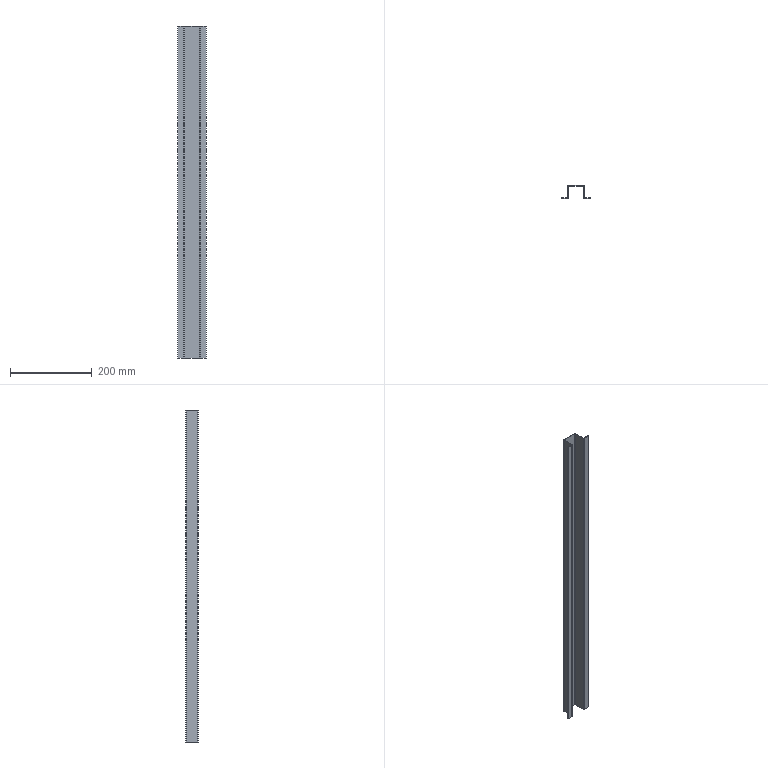Part | SolidWorks | features BaseBody 1 | 1 solid | 38 faces | box 70 x 31 x 812 mm | volume 103469 mm3 | plane 30 | cylinder 8 | commonest cylinder face diameters 2 x4 4 x4
STEP:
#1=CARTESIAN_POINT('',(41.,-1.,-406.));
#2=VERTEX_POINT('',#1);
#3=CARTESIAN_POINT('',(55.,-1.,-406.));
#4=VERTEX_POINT('',#3);
#5=CARTESIAN_POINT('',(40.,-1.,-406.));
#6=DIRECTION('',(1.,0.,0.));
#7=VECTOR('',#6,1000.);
#8=LINE('',#5,#7);
#9=EDGE_CURVE('',#2,#4,#8,.T.);
#10=ORIENTED_EDGE('',*,*,#9,.F.);
#11=CARTESIAN_POINT('',(41.,0.,-406.));
#12=VERTEX_POINT('',#11);
#13=CARTESIAN_POINT('',(41.,-1.,-406.));
#14=DIRECTION('',(0.,1.,0.));
#15=VECTOR('',#14,1000.);
#16=LINE('',#13,#15);
#17=EDGE_CURVE('',#2,#12,#16,.T.);
#18=ORIENTED_EDGE('',*,*,#17,.T.);
#19=CARTESIAN_POINT('',(55.,0.,-406.));
#20=VERTEX_POINT('',#19);
#21=CARTESIAN_POINT('',(40.,0.,-406.));
#22=DIRECTION('',(1.,0.,0.));
#23=VECTOR('',#22,1000.);
#24=LINE('',#21,#23);
#25=EDGE_CURVE('',#12,#20,#24,.T.);
#26=ORIENTED_EDGE('',*,*,#25,.T.);
#27=CARTESIAN_POINT('',(55.,0.,-406.));
#28=DIRECTION('',(0.,-1.,0.));
#29=VECTOR('',#28,1000.);
#30=LINE('',#27,#29);
#31=EDGE_CURVE('',#20,#4,#30,.T.);
#32=ORIENTED_EDGE('',*,*,#31,.T.);
#33=EDGE_LOOP('',(#10,#18,#26,#32));
#34=FACE_OUTER_BOUND('',#33,.T.);
#35=CARTESIAN_POINT('',(41.,1.,-406.));
#36=DIRECTION('',(0.,0.,-1.));
#37=DIRECTION('',(0.,-1.,0.));
#38=AXIS2_PLACEMENT_3D('',#35,#36,#37);
#39=PLANE('',#38);
#40=ADVANCED_FACE('',(#34),#39,.T.);
#41=CARTESIAN_POINT('',(-15.,-1.,406.));
#42=VERTEX_POINT('',#41);
#43=CARTESIAN_POINT('',(-1.,-1.,406.));
#44=VERTEX_POINT('',#43);
#45=CARTESIAN_POINT('',(0.,-1.,406.));
#46=DIRECTION('',(1.,0.,0.));
#47=VECTOR('',#46,1000.);
#48=LINE('',#45,#47);
#49=EDGE_CURVE('',#42,#44,#48,.T.);
#50=ORIENTED_EDGE('',*,*,#49,.T.);
#51=CARTESIAN_POINT('',(-1.,0.,406.));
#52=VERTEX_POINT('',#51);
#53=CARTESIAN_POINT('',(-1.,-1.,406.));
#54=DIRECTION('',(0.,1.,0.));
#55=VECTOR('',#54,1000.);
#56=LINE('',#53,#55);
#57=EDGE_CURVE('',#44,#52,#56,.T.);
#58=ORIENTED_EDGE('',*,*,#57,.T.);
#59=CARTESIAN_POINT('',(-15.,0.,406.));
#60=VERTEX_POINT('',#59);
#61=CARTESIAN_POINT('',(0.,0.,406.));
#62=DIRECTION('',(1.,0.,0.));
#63=VECTOR('',#62,1000.);
#64=LINE('',#61,#63);
#65=EDGE_CURVE('',#60,#52,#64,.T.);
#66=ORIENTED_EDGE('',*,*,#65,.F.);
#67=CARTESIAN_POINT('',(-15.,-1.,406.));
#68=DIRECTION('',(0.,1.,0.));
#69=VECTOR('',#68,1000.);
#70=LINE('',#67,#69);
#71=EDGE_CURVE('',#42,#60,#70,.T.);
#72=ORIENTED_EDGE('',*,*,#71,.F.);
#73=EDGE_LOOP('',(#50,#58,#66,#72));
#74=FACE_OUTER_BOUND('',#73,.T.);
#75=CARTESIAN_POINT('',(41.,1.,406.));
#76=DIRECTION('',(0.,0.,-1.));
#77=DIRECTION('',(0.,-1.,0.));
#78=AXIS2_PLACEMENT_3D('',#75,#76,#77);
#79=PLANE('',#78);
#80=ADVANCED_FACE('',(#74),#79,.F.);
#81=CARTESIAN_POINT('',(39.,1.,-406.));
#82=VERTEX_POINT('',#81);
#83=CARTESIAN_POINT('',(41.,1.,-406.));
#84=DIRECTION('',(0.,0.,1.));
#85=DIRECTION('',(1.,0.,0.));
#86=AXIS2_PLACEMENT_3D('',#83,#84,#85);
#87=CIRCLE('',#86,2.);
#88=EDGE_CURVE('',#82,#2,#87,.T.);
#89=ORIENTED_EDGE('',*,*,#88,.T.);
#90=CARTESIAN_POINT('',(41.,-1.,406.));
#91=VERTEX_POINT('',#90);
#92=CARTESIAN_POINT('',(41.,-1.,406.));
#93=DIRECTION('',(0.,0.,-1.));
#94=VECTOR('',#93,1000.);
#95=LINE('',#92,#94);
#96=EDGE_CURVE('',#91,#2,#95,.T.);
#97=ORIENTED_EDGE('',*,*,#96,.F.);
#98=CARTESIAN_POINT('',(39.,1.,406.));
#99=VERTEX_POINT('',#98);
#100=CARTESIAN_POINT('',(41.,1.,406.));
#101=DIRECTION('',(0.,0.,1.));
#102=DIRECTION('',(1.,0.,0.));
#103=AXIS2_PLACEMENT_3D('',#100,#101,#102);
#104=CIRCLE('',#103,2.);
#105=EDGE_CURVE('',#99,#91,#104,.T.);
#106=ORIENTED_EDGE('',*,*,#105,.F.);
#107=CARTESIAN_POINT('',(39.,1.,406.));
#108=DIRECTION('',(0.,0.,-1.));
#109=VECTOR('',#108,1000.);
#110=LINE('',#107,#109);
#111=EDGE_CURVE('',#99,#82,#110,.T.);
#112=ORIENTED_EDGE('',*,*,#111,.T.);
#113=EDGE_LOOP('',(#89,#97,#106,#112));
#114=FACE_OUTER_BOUND('',#113,.T.);
#115=CARTESIAN_POINT('',(41.,1.,406.));
#116=DIRECTION('',(0.,0.,-1.));
#117=DIRECTION('',(-1.,0.,0.));
#118=AXIS2_PLACEMENT_3D('',#115,#116,#117);
#119=CYLINDRICAL_SURFACE('',#118,2.);
#120=ADVANCED_FACE('',(#114),#119,.T.);
#121=CARTESIAN_POINT('',(39.,28.,-406.));
#122=VERTEX_POINT('',#121);
#123=CARTESIAN_POINT('',(39.,30.,-406.));
#124=DIRECTION('',(0.,-1.,0.));
#125=VECTOR('',#124,1000.);
#126=LINE('',#123,#125);
#127=EDGE_CURVE('',#122,#82,#126,.T.);
#128=ORIENTED_EDGE('',*,*,#127,.T.);
#129=ORIENTED_EDGE('',*,*,#111,.F.);
#130=CARTESIAN_POINT('',(39.,28.,406.));
#131=VERTEX_POINT('',#130);
#132=CARTESIAN_POINT('',(39.,30.,406.));
#133=DIRECTION('',(0.,-1.,0.));
#134=VECTOR('',#133,1000.);
#135=LINE('',#132,#134);
#136=EDGE_CURVE('',#131,#99,#135,.T.);
#137=ORIENTED_EDGE('',*,*,#136,.F.);
#138=CARTESIAN_POINT('',(39.,28.,406.));
#139=DIRECTION('',(0.,0.,-1.));
#140=VECTOR('',#139,1000.);
#141=LINE('',#138,#140);
#142=EDGE_CURVE('',#131,#122,#141,.T.);
#143=ORIENTED_EDGE('',*,*,#142,.T.);
#144=EDGE_LOOP('',(#128,#129,#137,#143));
#145=FACE_OUTER_BOUND('',#144,.T.);
#146=CARTESIAN_POINT('',(39.,30.,406.));
#147=DIRECTION('',(1.,0.,0.));
#148=DIRECTION('',(0.,1.,0.));
#149=AXIS2_PLACEMENT_3D('',#146,#147,#148);
#150=PLANE('',#149);
#151=ADVANCED_FACE('',(#145),#150,.F.);
#152=CARTESIAN_POINT('',(38.,29.,-406.));
#153=VERTEX_POINT('',#152);
#154=CARTESIAN_POINT('',(38.,28.,-406.));
#155=DIRECTION('',(0.,0.,-1.));
#156=DIRECTION('',(1.,0.,0.));
#157=AXIS2_PLACEMENT_3D('',#154,#155,#156);
#158=CIRCLE('',#157,1.);
#159=EDGE_CURVE('',#153,#122,#158,.T.);
#160=ORIENTED_EDGE('',*,*,#159,.T.);
#161=ORIENTED_EDGE('',*,*,#142,.F.);
#162=CARTESIAN_POINT('',(38.,29.,406.));
#163=VERTEX_POINT('',#162);
#164=CARTESIAN_POINT('',(38.,28.,406.));
#165=DIRECTION('',(0.,0.,-1.));
#166=DIRECTION('',(1.,0.,0.));
#167=AXIS2_PLACEMENT_3D('',#164,#165,#166);
#168=CIRCLE('',#167,1.);
#169=EDGE_CURVE('',#163,#131,#168,.T.);
#170=ORIENTED_EDGE('',*,*,#169,.F.);
#171=CARTESIAN_POINT('',(38.,29.,406.));
#172=DIRECTION('',(0.,0.,-1.));
#173=VECTOR('',#172,1000.);
#174=LINE('',#171,#173);
#175=EDGE_CURVE('',#163,#153,#174,.T.);
#176=ORIENTED_EDGE('',*,*,#175,.T.);
#177=EDGE_LOOP('',(#160,#161,#170,#176));
#178=FACE_OUTER_BOUND('',#177,.T.);
#179=CARTESIAN_POINT('',(38.,28.,406.));
#180=DIRECTION('',(0.,0.,-1.));
#181=DIRECTION('',(-1.,0.,0.));
#182=AXIS2_PLACEMENT_3D('',#179,#180,#181);
#183=CYLINDRICAL_SURFACE('',#182,1.);
#184=ADVANCED_FACE('',(#178),#183,.F.);
#185=CARTESIAN_POINT('',(2.,29.,-406.));
#186=VERTEX_POINT('',#185);
#187=CARTESIAN_POINT('',(0.,29.,-406.));
#188=DIRECTION('',(1.,0.,0.));
#189=VECTOR('',#188,1000.);
#190=LINE('',#187,#189);
#191=EDGE_CURVE('',#186,#153,#190,.T.);
#192=ORIENTED_EDGE('',*,*,#191,.T.);
#193=ORIENTED_EDGE('',*,*,#175,.F.);
#194=CARTESIAN_POINT('',(2.,29.,406.));
#195=VERTEX_POINT('',#194);
#196=CARTESIAN_POINT('',(0.,29.,406.));
#197=DIRECTION('',(1.,0.,0.));
#198=VECTOR('',#197,1000.);
#199=LINE('',#196,#198);
#200=EDGE_CURVE('',#195,#163,#199,.T.);
#201=ORIENTED_EDGE('',*,*,#200,.F.);
#202=CARTESIAN_POINT('',(2.,29.,406.));
#203=DIRECTION('',(0.,0.,-1.));
#204=VECTOR('',#203,1000.);
#205=LINE('',#202,#204);
#206=EDGE_CURVE('',#195,#186,#205,.T.);
#207=ORIENTED_EDGE('',*,*,#206,.T.);
#208=EDGE_LOOP('',(#192,#193,#201,#207));
#209=FACE_OUTER_BOUND('',#208,.T.);
#210=CARTESIAN_POINT('',(0.,29.,406.));
#211=DIRECTION('',(0.,1.,0.));
#212=DIRECTION('',(1.,0.,0.));
#213=AXIS2_PLACEMENT_3D('',#210,#211,#212);
#214=PLANE('',#213);
#215=ADVANCED_FACE('',(#209),#214,.F.);
#216=CARTESIAN_POINT('',(1.,28.,-406.));
#217=VERTEX_POINT('',#216);
#218=CARTESIAN_POINT('',(2.,28.,-406.));
#219=DIRECTION('',(0.,0.,-1.));
#220=DIRECTION('',(1.,0.,0.));
#221=AXIS2_PLACEMENT_3D('',#218,#219,#220);
#222=CIRCLE('',#221,1.);
#223=EDGE_CURVE('',#217,#186,#222,.T.);
#224=ORIENTED_EDGE('',*,*,#223,.T.);
#225=ORIENTED_EDGE('',*,*,#206,.F.);
#226=CARTESIAN_POINT('',(1.,28.,406.));
#227=VERTEX_POINT('',#226);
#228=CARTESIAN_POINT('',(2.,28.,406.));
#229=DIRECTION('',(0.,0.,-1.));
#230=DIRECTION('',(1.,0.,0.));
#231=AXIS2_PLACEMENT_3D('',#228,#229,#230);
#232=CIRCLE('',#231,1.);
#233=EDGE_CURVE('',#227,#195,#232,.T.);
#234=ORIENTED_EDGE('',*,*,#233,.F.);
#235=CARTESIAN_POINT('',(1.,28.,406.));
#236=DIRECTION('',(0.,0.,-1.));
#237=VECTOR('',#236,1000.);
#238=LINE('',#235,#237);
#239=EDGE_CURVE('',#227,#217,#238,.T.);
#240=ORIENTED_EDGE('',*,*,#239,.T.);
#241=EDGE_LOOP('',(#224,#225,#234,#240));
#242=FACE_OUTER_BOUND('',#241,.T.);
#243=CARTESIAN_POINT('',(2.,28.,406.));
#244=DIRECTION('',(0.,0.,-1.));
#245=DIRECTION('',(-1.,0.,0.));
#246=AXIS2_PLACEMENT_3D('',#243,#244,#245);
#247=CYLINDRICAL_SURFACE('',#246,1.);
#248=ADVANCED_FACE('',(#242),#247,.F.);
#249=CARTESIAN_POINT('',(1.,1.,-406.));
#250=VERTEX_POINT('',#249);
#251=CARTESIAN_POINT('',(1.,0.,-406.));
#252=DIRECTION('',(0.,1.,0.));
#253=VECTOR('',#252,1000.);
#254=LINE('',#251,#253);
#255=EDGE_CURVE('',#250,#217,#254,.T.);
#256=ORIENTED_EDGE('',*,*,#255,.T.);
#257=ORIENTED_EDGE('',*,*,#239,.F.);
#258=CARTESIAN_POINT('',(1.,1.,406.));
#259=VERTEX_POINT('',#258);
#260=CARTESIAN_POINT('',(1.,0.,406.));
#261=DIRECTION('',(0.,1.,0.));
#262=VECTOR('',#261,1000.);
#263=LINE('',#260,#262);
#264=EDGE_CURVE('',#259,#227,#263,.T.);
#265=ORIENTED_EDGE('',*,*,#264,.F.);
#266=CARTESIAN_POINT('',(1.,1.,406.));
#267=DIRECTION('',(0.,0.,-1.));
#268=VECTOR('',#267,1000.);
#269=LINE('',#266,#268);
#270=EDGE_CURVE('',#259,#250,#269,.T.);
#271=ORIENTED_EDGE('',*,*,#270,.T.);
#272=EDGE_LOOP('',(#256,#257,#265,#271));
#273=FACE_OUTER_BOUND('',#272,.T.);
#274=CARTESIAN_POINT('',(1.,0.,406.));
#275=DIRECTION('',(-1.,0.,0.));
#276=DIRECTION('',(0.,0.,1.));
#277=AXIS2_PLACEMENT_3D('',#274,#275,#276);
#278=PLANE('',#277);
#279=ADVANCED_FACE('',(#273),#278,.F.);
#280=CARTESIAN_POINT('',(-1.,-1.,-406.));
#281=VERTEX_POINT('',#280);
#282=CARTESIAN_POINT('',(-1.,1.,-406.));
#283=DIRECTION('',(0.,0.,1.));
#284=DIRECTION('',(1.,0.,0.));
#285=AXIS2_PLACEMENT_3D('',#282,#283,#284);
#286=CIRCLE('',#285,2.);
#287=EDGE_CURVE('',#281,#250,#286,.T.);
#288=ORIENTED_EDGE('',*,*,#287,.T.);
#289=ORIENTED_EDGE('',*,*,#270,.F.);
#290=CARTESIAN_POINT('',(-1.,1.,406.));
#291=DIRECTION('',(0.,0.,1.));
#292=DIRECTION('',(1.,0.,0.));
#293=AXIS2_PLACEMENT_3D('',#290,#291,#292);
#294=CIRCLE('',#293,2.);
#295=EDGE_CURVE('',#44,#259,#294,.T.);
#296=ORIENTED_EDGE('',*,*,#295,.F.);
#297=CARTESIAN_POINT('',(-1.,-1.,406.));
#298=DIRECTION('',(0.,0.,-1.));
#299=VECTOR('',#298,1000.);
#300=LINE('',#297,#299);
#301=EDGE_CURVE('',#44,#281,#300,.T.);
#302=ORIENTED_EDGE('',*,*,#301,.T.);
#303=EDGE_LOOP('',(#288,#289,#296,#302));
#304=FACE_OUTER_BOUND('',#303,.T.);
#305=CARTESIAN_POINT('',(-1.,1.,406.));
#306=DIRECTION('',(0.,0.,-1.));
#307=DIRECTION('',(-1.,0.,0.));
#308=AXIS2_PLACEMENT_3D('',#305,#306,#307);
#309=CYLINDRICAL_SURFACE('',#308,2.);
#310=ADVANCED_FACE('',(#304),#309,.T.);
#311=CARTESIAN_POINT('',(-15.,-1.,-406.));
#312=VERTEX_POINT('',#311);
#313=CARTESIAN_POINT('',(0.,-1.,-406.));
#314=DIRECTION('',(1.,0.,0.));
#315=VECTOR('',#314,1000.);
#316=LINE('',#313,#315);
#317=EDGE_CURVE('',#312,#281,#316,.T.);
#318=ORIENTED_EDGE('',*,*,#317,.T.);
#319=ORIENTED_EDGE('',*,*,#301,.F.);
#320=ORIENTED_EDGE('',*,*,#49,.F.);
#321=CARTESIAN_POINT('',(-15.,-1.,406.));
#322=DIRECTION('',(0.,0.,-1.));
#323=VECTOR('',#322,1000.);
#324=LINE('',#321,#323);
#325=EDGE_CURVE('',#42,#312,#324,.T.);
#326=ORIENTED_EDGE('',*,*,#325,.T.);
#327=EDGE_LOOP('',(#318,#319,#320,#326));
#328=FACE_OUTER_BOUND('',#327,.T.);
#329=CARTESIAN_POINT('',(0.,-1.,406.));
#330=DIRECTION('',(0.,1.,0.));
#331=DIRECTION('',(1.,0.,0.));
#332=AXIS2_PLACEMENT_3D('',#329,#330,#331);
#333=PLANE('',#332);
#334=ADVANCED_FACE('',(#328),#333,.F.);
#335=CARTESIAN_POINT('',(-15.,0.,-406.));
#336=VERTEX_POINT('',#335);
#337=CARTESIAN_POINT('',(-15.,-1.,-406.));
#338=DIRECTION('',(0.,1.,0.));
#339=VECTOR('',#338,1000.);
#340=LINE('',#337,#339);
#341=EDGE_CURVE('',#312,#336,#340,.T.);
#342=ORIENTED_EDGE('',*,*,#341,.F.);
#343=ORIENTED_EDGE('',*,*,#325,.F.);
#344=ORIENTED_EDGE('',*,*,#71,.T.);
#345=CARTESIAN_POINT('',(-15.,0.,406.));
#346=DIRECTION('',(0.,0.,-1.));
#347=VECTOR('',#346,1000.);
#348=LINE('',#345,#347);
#349=EDGE_CURVE('',#60,#336,#348,.T.);
#350=ORIENTED_EDGE('',*,*,#349,.T.);
#351=EDGE_LOOP('',(#342,#343,#344,#350));
#352=FACE_OUTER_BOUND('',#351,.T.);
#353=CARTESIAN_POINT('',(-15.,-1.,406.));
#354=DIRECTION('',(-1.,0.,0.));
#355=DIRECTION('',(0.,0.,1.));
#356=AXIS2_PLACEMENT_3D('',#353,#354,#355);
#357=PLANE('',#356);
#358=ADVANCED_FACE('',(#352),#357,.T.);
#359=CARTESIAN_POINT('',(-1.,0.,-406.));
#360=VERTEX_POINT('',#359);
#361=CARTESIAN_POINT('',(0.,0.,-406.));
#362=DIRECTION('',(1.,0.,0.));
#363=VECTOR('',#362,1000.);
#364=LINE('',#361,#363);
#365=EDGE_CURVE('',#336,#360,#364,.T.);
#366=ORIENTED_EDGE('',*,*,#365,.F.);
#367=ORIENTED_EDGE('',*,*,#349,.F.);
#368=ORIENTED_EDGE('',*,*,#65,.T.);
#369=CARTESIAN_POINT('',(-1.,0.,406.));
#370=DIRECTION('',(0.,0.,-1.));
#371=VECTOR('',#370,1000.);
#372=LINE('',#369,#371);
#373=EDGE_CURVE('',#52,#360,#372,.T.);
#374=ORIENTED_EDGE('',*,*,#373,.T.);
#375=EDGE_LOOP('',(#366,#367,#368,#374));
#376=FACE_OUTER_BOUND('',#375,.T.);
#377=CARTESIAN_POINT('',(0.,0.,406.));
#378=DIRECTION('',(0.,1.,0.));
#379=DIRECTION('',(1.,0.,0.));
#380=AXIS2_PLACEMENT_3D('',#377,#378,#379);
#381=PLANE('',#380);
#382=ADVANCED_FACE('',(#376),#381,.T.);
#383=CARTESIAN_POINT('',(0.,1.,-406.));
#384=VERTEX_POINT('',#383);
#385=CARTESIAN_POINT('',(-1.,1.,-406.));
#386=DIRECTION('',(0.,0.,1.));
#387=DIRECTION('',(-1.,0.,0.));
#388=AXIS2_PLACEMENT_3D('',#385,#386,#387);
#389=CIRCLE('',#388,1.);
#390=EDGE_CURVE('',#360,#384,#389,.T.);
#391=ORIENTED_EDGE('',*,*,#390,.F.);
#392=ORIENTED_EDGE('',*,*,#373,.F.);
#393=CARTESIAN_POINT('',(0.,1.,406.));
#394=VERTEX_POINT('',#393);
#395=CARTESIAN_POINT('',(-1.,1.,406.));
#396=DIRECTION('',(0.,0.,1.));
#397=DIRECTION('',(-1.,0.,0.));
#398=AXIS2_PLACEMENT_3D('',#395,#396,#397);
#399=CIRCLE('',#398,1.);
#400=EDGE_CURVE('',#52,#394,#399,.T.);
#401=ORIENTED_EDGE('',*,*,#400,.T.);
#402=CARTESIAN_POINT('',(0.,1.,406.));
#403=DIRECTION('',(0.,0.,-1.));
#404=VECTOR('',#403,1000.);
#405=LINE('',#402,#404);
#406=EDGE_CURVE('',#394,#384,#405,.T.);
#407=ORIENTED_EDGE('',*,*,#406,.T.);
#408=EDGE_LOOP('',(#391,#392,#401,#407));
#409=FACE_OUTER_BOUND('',#408,.T.);
#410=CARTESIAN_POINT('',(-1.,1.,406.));
#411=DIRECTION('',(0.,0.,-1.));
#412=DIRECTION('',(-1.,0.,0.));
#413=AXIS2_PLACEMENT_3D('',#410,#411,#412);
#414=CYLINDRICAL_SURFACE('',#413,1.);
#415=ADVANCED_FACE('',(#409),#414,.F.);
#416=CARTESIAN_POINT('',(0.,28.,-406.));
#417=VERTEX_POINT('',#416);
#418=CARTESIAN_POINT('',(0.,0.,-406.));
#419=DIRECTION('',(0.,1.,0.));
#420=VECTOR('',#419,1000.);
#421=LINE('',#418,#420);
#422=EDGE_CURVE('',#384,#417,#421,.T.);
#423=ORIENTED_EDGE('',*,*,#422,.F.);
#424=ORIENTED_EDGE('',*,*,#406,.F.);
#425=CARTESIAN_POINT('',(0.,28.,406.));
#426=VERTEX_POINT('',#425);
#427=CARTESIAN_POINT('',(0.,0.,406.));
#428=DIRECTION('',(0.,1.,0.));
#429=VECTOR('',#428,1000.);
#430=LINE('',#427,#429);
#431=EDGE_CURVE('',#394,#426,#430,.T.);
#432=ORIENTED_EDGE('',*,*,#431,.T.);
#433=CARTESIAN_POINT('',(0.,28.,406.));
#434=DIRECTION('',(0.,0.,-1.));
#435=VECTOR('',#434,1000.);
#436=LINE('',#433,#435);
#437=EDGE_CURVE('',#426,#417,#436,.T.);
#438=ORIENTED_EDGE('',*,*,#437,.T.);
#439=EDGE_LOOP('',(#423,#424,#432,#438));
#440=FACE_OUTER_BOUND('',#439,.T.);
#441=CARTESIAN_POINT('',(0.,0.,406.));
#442=DIRECTION('',(-1.,0.,0.));
#443=DIRECTION('',(0.,0.,1.));
#444=AXIS2_PLACEMENT_3D('',#441,#442,#443);
#445=PLANE('',#444);
#446=ADVANCED_FACE('',(#440),#445,.T.);
#447=CARTESIAN_POINT('',(2.,30.,-406.));
#448=VERTEX_POINT('',#447);
#449=CARTESIAN_POINT('',(2.,28.,-406.));
#450=DIRECTION('',(0.,0.,-1.));
#451=DIRECTION('',(1.,0.,0.));
#452=AXIS2_PLACEMENT_3D('',#449,#450,#451);
#453=CIRCLE('',#452,2.);
#454=EDGE_CURVE('',#417,#448,#453,.T.);
#455=ORIENTED_EDGE('',*,*,#454,.F.);
#456=ORIENTED_EDGE('',*,*,#437,.F.);
#457=CARTESIAN_POINT('',(2.,30.,406.));
#458=VERTEX_POINT('',#457);
#459=CARTESIAN_POINT('',(2.,28.,406.));
#460=DIRECTION('',(0.,0.,-1.));
#461=DIRECTION('',(1.,0.,0.));
#462=AXIS2_PLACEMENT_3D('',#459,#460,#461);
#463=CIRCLE('',#462,2.);
#464=EDGE_CURVE('',#426,#458,#463,.T.);
#465=ORIENTED_EDGE('',*,*,#464,.T.);
#466=CARTESIAN_POINT('',(2.,30.,406.));
#467=DIRECTION('',(0.,0.,-1.));
#468=VECTOR('',#467,1000.);
#469=LINE('',#466,#468);
#470=EDGE_CURVE('',#458,#448,#469,.T.);
#471=ORIENTED_EDGE('',*,*,#470,.T.);
#472=EDGE_LOOP('',(#455,#456,#465,#471));
#473=FACE_OUTER_BOUND('',#472,.T.);
#474=CARTESIAN_POINT('',(2.,28.,406.));
#475=DIRECTION('',(0.,0.,-1.));
#476=DIRECTION('',(-1.,0.,0.));
#477=AXIS2_PLACEMENT_3D('',#474,#475,#476);
#478=CYLINDRICAL_SURFACE('',#477,2.);
#479=ADVANCED_FACE('',(#473),#478,.T.);
#480=CARTESIAN_POINT('',(38.,30.,-406.));
#481=VERTEX_POINT('',#480);
#482=CARTESIAN_POINT('',(0.,30.,-406.));
#483=DIRECTION('',(1.,0.,0.));
#484=VECTOR('',#483,1000.);
#485=LINE('',#482,#484);
#486=EDGE_CURVE('',#448,#481,#485,.T.);
#487=ORIENTED_EDGE('',*,*,#486,.F.);
#488=ORIENTED_EDGE('',*,*,#470,.F.);
#489=CARTESIAN_POINT('',(38.,30.,406.));
#490=VERTEX_POINT('',#489);
#491=CARTESIAN_POINT('',(0.,30.,406.));
#492=DIRECTION('',(1.,0.,0.));
#493=VECTOR('',#492,1000.);
#494=LINE('',#491,#493);
#495=EDGE_CURVE('',#458,#490,#494,.T.);
#496=ORIENTED_EDGE('',*,*,#495,.T.);
#497=CARTESIAN_POINT('',(38.,30.,406.));
#498=DIRECTION('',(0.,0.,-1.));
#499=VECTOR('',#498,1000.);
#500=LINE('',#497,#499);
#501=EDGE_CURVE('',#490,#481,#500,.T.);
#502=ORIENTED_EDGE('',*,*,#501,.T.);
#503=EDGE_LOOP('',(#487,#488,#496,#502));
#504=FACE_OUTER_BOUND('',#503,.T.);
#505=CARTESIAN_POINT('',(0.,30.,406.));
#506=DIRECTION('',(0.,1.,0.));
#507=DIRECTION('',(1.,0.,0.));
#508=AXIS2_PLACEMENT_3D('',#505,#506,#507);
#509=PLANE('',#508);
#510=ADVANCED_FACE('',(#504),#509,.T.);
#511=CARTESIAN_POINT('',(40.,28.,-406.));
#512=VERTEX_POINT('',#511);
#513=CARTESIAN_POINT('',(38.,28.,-406.));
#514=DIRECTION('',(0.,0.,-1.));
#515=DIRECTION('',(1.,0.,0.));
#516=AXIS2_PLACEMENT_3D('',#513,#514,#515);
#517=CIRCLE('',#516,2.);
#518=EDGE_CURVE('',#481,#512,#517,.T.);
#519=ORIENTED_EDGE('',*,*,#518,.F.);
#520=ORIENTED_EDGE('',*,*,#501,.F.);
#521=CARTESIAN_POINT('',(40.,28.,406.));
#522=VERTEX_POINT('',#521);
#523=CARTESIAN_POINT('',(38.,28.,406.));
#524=DIRECTION('',(0.,0.,-1.));
#525=DIRECTION('',(1.,0.,0.));
#526=AXIS2_PLACEMENT_3D('',#523,#524,#525);
#527=CIRCLE('',#526,2.);
#528=EDGE_CURVE('',#490,#522,#527,.T.);
#529=ORIENTED_EDGE('',*,*,#528,.T.);
#530=CARTESIAN_POINT('',(40.,28.,406.));
#531=DIRECTION('',(0.,0.,-1.));
#532=VECTOR('',#531,1000.);
#533=LINE('',#530,#532);
#534=EDGE_CURVE('',#522,#512,#533,.T.);
#535=ORIENTED_EDGE('',*,*,#534,.T.);
#536=EDGE_LOOP('',(#519,#520,#529,#535));
#537=FACE_OUTER_BOUND('',#536,.T.);
#538=CARTESIAN_POINT('',(38.,28.,406.));
#539=DIRECTION('',(0.,0.,-1.));
#540=DIRECTION('',(-1.,0.,0.));
#541=AXIS2_PLACEMENT_3D('',#538,#539,#540);
#542=CYLINDRICAL_SURFACE('',#541,2.);
#543=ADVANCED_FACE('',(#537),#542,.T.);
#544=CARTESIAN_POINT('',(40.,1.,-406.));
#545=VERTEX_POINT('',#544);
#546=CARTESIAN_POINT('',(40.,30.,-406.));
#547=DIRECTION('',(0.,-1.,0.));
#548=VECTOR('',#547,1000.);
#549=LINE('',#546,#548);
#550=EDGE_CURVE('',#512,#545,#549,.T.);
#551=ORIENTED_EDGE('',*,*,#550,.F.);
#552=ORIENTED_EDGE('',*,*,#534,.F.);
#553=CARTESIAN_POINT('',(40.,1.,406.));
#554=VERTEX_POINT('',#553);
#555=CARTESIAN_POINT('',(40.,30.,406.));
#556=DIRECTION('',(0.,-1.,0.));
#557=VECTOR('',#556,1000.);
#558=LINE('',#555,#557);
#559=EDGE_CURVE('',#522,#554,#558,.T.);
#560=ORIENTED_EDGE('',*,*,#559,.T.);
#561=CARTESIAN_POINT('',(40.,1.,406.));
#562=DIRECTION('',(0.,0.,-1.));
#563=VECTOR('',#562,1000.);
#564=LINE('',#561,#563);
#565=EDGE_CURVE('',#554,#545,#564,.T.);
#566=ORIENTED_EDGE('',*,*,#565,.T.);
#567=EDGE_LOOP('',(#551,#552,#560,#566));
#568=FACE_OUTER_BOUND('',#567,.T.);
#569=CARTESIAN_POINT('',(40.,30.,406.));
#570=DIRECTION('',(1.,0.,0.));
#571=DIRECTION('',(0.,1.,0.));
#572=AXIS2_PLACEMENT_3D('',#569,#570,#571);
#573=PLANE('',#572);
#574=ADVANCED_FACE('',(#568),#573,.T.);
#575=CARTESIAN_POINT('',(41.,1.,-406.));
#576=DIRECTION('',(0.,0.,1.));
#577=DIRECTION('',(-1.,0.,0.));
#578=AXIS2_PLACEMENT_3D('',#575,#576,#577);
#579=CIRCLE('',#578,1.);
#580=EDGE_CURVE('',#545,#12,#579,.T.);
#581=ORIENTED_EDGE('',*,*,#580,.F.);
#582=ORIENTED_EDGE('',*,*,#565,.F.);
#583=CARTESIAN_POINT('',(41.,0.,406.));
#584=VERTEX_POINT('',#583);
#585=CARTESIAN_POINT('',(41.,1.,406.));
#586=DIRECTION('',(0.,0.,1.));
#587=DIRECTION('',(-1.,0.,0.));
#588=AXIS2_PLACEMENT_3D('',#585,#586,#587);
#589=CIRCLE('',#588,1.);
#590=EDGE_CURVE('',#554,#584,#589,.T.);
#591=ORIENTED_EDGE('',*,*,#590,.T.);
#592=CARTESIAN_POINT('',(41.,0.,406.));
#593=DIRECTION('',(0.,0.,-1.));
#594=VECTOR('',#593,1000.);
#595=LINE('',#592,#594);
#596=EDGE_CURVE('',#584,#12,#595,.T.);
#597=ORIENTED_EDGE('',*,*,#596,.T.);
#598=EDGE_LOOP('',(#581,#582,#591,#597));
#599=FACE_OUTER_BOUND('',#598,.T.);
#600=CARTESIAN_POINT('',(41.,1.,406.));
#601=DIRECTION('',(0.,0.,-1.));
#602=DIRECTION('',(-1.,0.,0.));
#603=AXIS2_PLACEMENT_3D('',#600,#601,#602);
#604=CYLINDRICAL_SURFACE('',#603,1.);
#605=ADVANCED_FACE('',(#599),#604,.F.);
#606=ORIENTED_EDGE('',*,*,#25,.F.);
#607=ORIENTED_EDGE('',*,*,#596,.F.);
#608=CARTESIAN_POINT('',(55.,0.,406.));
#609=VERTEX_POINT('',#608);
#610=CARTESIAN_POINT('',(40.,0.,406.));
#611=DIRECTION('',(1.,0.,0.));
#612=VECTOR('',#611,1000.);
#613=LINE('',#610,#612);
#614=EDGE_CURVE('',#584,#609,#613,.T.);
#615=ORIENTED_EDGE('',*,*,#614,.T.);
#616=CARTESIAN_POINT('',(55.,0.,406.));
#617=DIRECTION('',(0.,0.,-1.));
#618=VECTOR('',#617,1000.);
#619=LINE('',#616,#618);
#620=EDGE_CURVE('',#609,#20,#619,.T.);
#621=ORIENTED_EDGE('',*,*,#620,.T.);
#622=EDGE_LOOP('',(#606,#607,#615,#621));
#623=FACE_OUTER_BOUND('',#622,.T.);
#624=CARTESIAN_POINT('',(40.,0.,406.));
#625=DIRECTION('',(0.,1.,0.));
#626=DIRECTION('',(1.,0.,0.));
#627=AXIS2_PLACEMENT_3D('',#624,#625,#626);
#628=PLANE('',#627);
#629=ADVANCED_FACE('',(#623),#628,.T.);
#630=ORIENTED_EDGE('',*,*,#31,.F.);
#631=ORIENTED_EDGE('',*,*,#620,.F.);
#632=CARTESIAN_POINT('',(55.,-1.,406.));
#633=VERTEX_POINT('',#632);
#634=CARTESIAN_POINT('',(55.,0.,406.));
#635=DIRECTION('',(0.,-1.,0.));
#636=VECTOR('',#635,1000.);
#637=LINE('',#634,#636);
#638=EDGE_CURVE('',#609,#633,#637,.T.);
#639=ORIENTED_EDGE('',*,*,#638,.T.);
#640=CARTESIAN_POINT('',(55.,-1.,406.));
#641=DIRECTION('',(0.,0.,-1.));
#642=VECTOR('',#641,1000.);
#643=LINE('',#640,#642);
#644=EDGE_CURVE('',#633,#4,#643,.T.);
#645=ORIENTED_EDGE('',*,*,#644,.T.);
#646=EDGE_LOOP('',(#630,#631,#639,#645));
#647=FACE_OUTER_BOUND('',#646,.T.);
#648=CARTESIAN_POINT('',(55.,0.,406.));
#649=DIRECTION('',(1.,0.,0.));
#650=DIRECTION('',(0.,1.,0.));
#651=AXIS2_PLACEMENT_3D('',#648,#649,#650);
#652=PLANE('',#651);
#653=ADVANCED_FACE('',(#647),#652,.T.);
#654=ORIENTED_EDGE('',*,*,#9,.T.);
#655=ORIENTED_EDGE('',*,*,#644,.F.);
#656=CARTESIAN_POINT('',(40.,-1.,406.));
#657=DIRECTION('',(1.,0.,0.));
#658=VECTOR('',#657,1000.);
#659=LINE('',#656,#658);
#660=EDGE_CURVE('',#91,#633,#659,.T.);
#661=ORIENTED_EDGE('',*,*,#660,.F.);
#662=ORIENTED_EDGE('',*,*,#96,.T.);
#663=EDGE_LOOP('',(#654,#655,#661,#662));
#664=FACE_OUTER_BOUND('',#663,.T.);
#665=CARTESIAN_POINT('',(40.,-1.,406.));
#666=DIRECTION('',(0.,1.,0.));
#667=DIRECTION('',(1.,0.,0.));
#668=AXIS2_PLACEMENT_3D('',#665,#666,#667);
#669=PLANE('',#668);
#670=ADVANCED_FACE('',(#664),#669,.F.);
#671=ORIENTED_EDGE('',*,*,#550,.T.);
#672=CARTESIAN_POINT('',(40.,1.,-406.));
#673=DIRECTION('',(-1.,0.,0.));
#674=VECTOR('',#673,1000.);
#675=LINE('',#672,#674);
#676=EDGE_CURVE('',#545,#82,#675,.T.);
#677=ORIENTED_EDGE('',*,*,#676,.T.);
#678=ORIENTED_EDGE('',*,*,#127,.F.);
#679=CARTESIAN_POINT('',(39.,28.,-406.));
#680=DIRECTION('',(1.,0.,0.));
#681=VECTOR('',#680,1000.);
#682=LINE('',#679,#681);
#683=EDGE_CURVE('',#122,#512,#682,.T.);
#684=ORIENTED_EDGE('',*,*,#683,.T.);
#685=EDGE_LOOP('',(#671,#677,#678,#684));
#686=FACE_OUTER_BOUND('',#685,.T.);
#687=CARTESIAN_POINT('',(41.,-1.,-406.));
#688=DIRECTION('',(0.,0.,-1.));
#689=DIRECTION('',(0.,-1.,0.));
#690=AXIS2_PLACEMENT_3D('',#687,#688,#689);
#691=PLANE('',#690);
#692=ADVANCED_FACE('',(#686),#691,.T.);
#693=ORIENTED_EDGE('',*,*,#676,.F.);
#694=ORIENTED_EDGE('',*,*,#580,.T.);
#695=ORIENTED_EDGE('',*,*,#17,.F.);
#696=ORIENTED_EDGE('',*,*,#88,.F.);
#697=EDGE_LOOP('',(#693,#694,#695,#696));
#698=FACE_OUTER_BOUND('',#697,.T.);
#699=CARTESIAN_POINT('',(40.,1.,-406.));
#700=DIRECTION('',(0.,0.,-1.));
#701=DIRECTION('',(0.,-1.,0.));
#702=AXIS2_PLACEMENT_3D('',#699,#700,#701);
#703=PLANE('',#702);
#704=ADVANCED_FACE('',(#698),#703,.T.);
#705=ORIENTED_EDGE('',*,*,#614,.F.);
#706=CARTESIAN_POINT('',(41.,0.,406.));
#707=DIRECTION('',(0.,-1.,0.));
#708=VECTOR('',#707,1000.);
#709=LINE('',#706,#708);
#710=EDGE_CURVE('',#584,#91,#709,.T.);
#711=ORIENTED_EDGE('',*,*,#710,.T.);
#712=ORIENTED_EDGE('',*,*,#660,.T.);
#713=ORIENTED_EDGE('',*,*,#638,.F.);
#714=EDGE_LOOP('',(#705,#711,#712,#713));
#715=FACE_OUTER_BOUND('',#714,.T.);
#716=CARTESIAN_POINT('',(39.,1.,406.));
#717=DIRECTION('',(0.,0.,1.));
#718=DIRECTION('',(1.,0.,0.));
#719=AXIS2_PLACEMENT_3D('',#716,#717,#718);
#720=PLANE('',#719);
#721=ADVANCED_FACE('',(#715),#720,.T.);
#722=ORIENTED_EDGE('',*,*,#710,.F.);
#723=ORIENTED_EDGE('',*,*,#590,.F.);
#724=CARTESIAN_POINT('',(39.,1.,406.));
#725=DIRECTION('',(1.,0.,0.));
#726=VECTOR('',#725,1000.);
#727=LINE('',#724,#726);
#728=EDGE_CURVE('',#99,#554,#727,.T.);
#729=ORIENTED_EDGE('',*,*,#728,.F.);
#730=ORIENTED_EDGE('',*,*,#105,.T.);
#731=EDGE_LOOP('',(#722,#723,#729,#730));
#732=FACE_OUTER_BOUND('',#731,.T.);
#733=CARTESIAN_POINT('',(41.,0.,406.));
#734=DIRECTION('',(0.,0.,1.));
#735=DIRECTION('',(1.,0.,0.));
#736=AXIS2_PLACEMENT_3D('',#733,#734,#735);
#737=PLANE('',#736);
#738=ADVANCED_FACE('',(#732),#737,.T.);
#739=ORIENTED_EDGE('',*,*,#486,.T.);
#740=CARTESIAN_POINT('',(38.,30.,-406.));
#741=DIRECTION('',(0.,-1.,0.));
#742=VECTOR('',#741,1000.);
#743=LINE('',#740,#742);
#744=EDGE_CURVE('',#481,#153,#743,.T.);
#745=ORIENTED_EDGE('',*,*,#744,.T.);
#746=ORIENTED_EDGE('',*,*,#191,.F.);
#747=CARTESIAN_POINT('',(2.,29.,-406.));
#748=DIRECTION('',(0.,1.,0.));
#749=VECTOR('',#748,1000.);
#750=LINE('',#747,#749);
#751=EDGE_CURVE('',#186,#448,#750,.T.);
#752=ORIENTED_EDGE('',*,*,#751,.T.);
#753=EDGE_LOOP('',(#739,#745,#746,#752));
#754=FACE_OUTER_BOUND('',#753,.T.);
#755=CARTESIAN_POINT('',(39.,28.,-406.));
#756=DIRECTION('',(0.,0.,-1.));
#757=DIRECTION('',(0.,-1.,0.));
#758=AXIS2_PLACEMENT_3D('',#755,#756,#757);
#759=PLANE('',#758);
#760=ADVANCED_FACE('',(#754),#759,.T.);
#761=ORIENTED_EDGE('',*,*,#744,.F.);
#762=ORIENTED_EDGE('',*,*,#518,.T.);
#763=ORIENTED_EDGE('',*,*,#683,.F.);
#764=ORIENTED_EDGE('',*,*,#159,.F.);
#765=EDGE_LOOP('',(#761,#762,#763,#764));
#766=FACE_OUTER_BOUND('',#765,.T.);
#767=CARTESIAN_POINT('',(38.,30.,-406.));
#768=DIRECTION('',(0.,0.,-1.));
#769=DIRECTION('',(0.,-1.,0.));
#770=AXIS2_PLACEMENT_3D('',#767,#768,#769);
#771=PLANE('',#770);
#772=ADVANCED_FACE('',(#766),#771,.T.);
#773=ORIENTED_EDGE('',*,*,#559,.F.);
#774=CARTESIAN_POINT('',(40.,28.,406.));
#775=DIRECTION('',(-1.,0.,0.));
#776=VECTOR('',#775,1000.);
#777=LINE('',#774,#776);
#778=EDGE_CURVE('',#522,#131,#777,.T.);
#779=ORIENTED_EDGE('',*,*,#778,.T.);
#780=ORIENTED_EDGE('',*,*,#136,.T.);
#781=ORIENTED_EDGE('',*,*,#728,.T.);
#782=EDGE_LOOP('',(#773,#779,#780,#781));
#783=FACE_OUTER_BOUND('',#782,.T.);
#784=CARTESIAN_POINT('',(38.,29.,406.));
#785=DIRECTION('',(0.,0.,1.));
#786=DIRECTION('',(1.,0.,0.));
#787=AXIS2_PLACEMENT_3D('',#784,#785,#786);
#788=PLANE('',#787);
#789=ADVANCED_FACE('',(#783),#788,.T.);
#790=ORIENTED_EDGE('',*,*,#778,.F.);
#791=ORIENTED_EDGE('',*,*,#528,.F.);
#792=CARTESIAN_POINT('',(38.,29.,406.));
#793=DIRECTION('',(0.,1.,0.));
#794=VECTOR('',#793,1000.);
#795=LINE('',#792,#794);
#796=EDGE_CURVE('',#163,#490,#795,.T.);
#797=ORIENTED_EDGE('',*,*,#796,.F.);
#798=ORIENTED_EDGE('',*,*,#169,.T.);
#799=EDGE_LOOP('',(#790,#791,#797,#798));
#800=FACE_OUTER_BOUND('',#799,.T.);
#801=CARTESIAN_POINT('',(40.,28.,406.));
#802=DIRECTION('',(0.,0.,1.));
#803=DIRECTION('',(1.,0.,0.));
#804=AXIS2_PLACEMENT_3D('',#801,#802,#803);
#805=PLANE('',#804);
#806=ADVANCED_FACE('',(#800),#805,.T.);
#807=ORIENTED_EDGE('',*,*,#422,.T.);
#808=CARTESIAN_POINT('',(0.,28.,-406.));
#809=DIRECTION('',(1.,0.,0.));
#810=VECTOR('',#809,1000.);
#811=LINE('',#808,#810);
#812=EDGE_CURVE('',#417,#217,#811,.T.);
#813=ORIENTED_EDGE('',*,*,#812,.T.);
#814=ORIENTED_EDGE('',*,*,#255,.F.);
#815=CARTESIAN_POINT('',(1.,1.,-406.));
#816=DIRECTION('',(-1.,0.,0.));
#817=VECTOR('',#816,1000.);
#818=LINE('',#815,#817);
#819=EDGE_CURVE('',#250,#384,#818,.T.);
#820=ORIENTED_EDGE('',*,*,#819,.T.);
#821=EDGE_LOOP('',(#807,#813,#814,#820));
#822=FACE_OUTER_BOUND('',#821,.T.);
#823=CARTESIAN_POINT('',(2.,29.,-406.));
#824=DIRECTION('',(0.,0.,-1.));
#825=DIRECTION('',(0.,-1.,0.));
#826=AXIS2_PLACEMENT_3D('',#823,#824,#825);
#827=PLANE('',#826);
#828=ADVANCED_FACE('',(#822),#827,.T.);
#829=ORIENTED_EDGE('',*,*,#812,.F.);
#830=ORIENTED_EDGE('',*,*,#454,.T.);
#831=ORIENTED_EDGE('',*,*,#751,.F.);
#832=ORIENTED_EDGE('',*,*,#223,.F.);
#833=EDGE_LOOP('',(#829,#830,#831,#832));
#834=FACE_OUTER_BOUND('',#833,.T.);
#835=CARTESIAN_POINT('',(0.,28.,-406.));
#836=DIRECTION('',(0.,0.,-1.));
#837=DIRECTION('',(0.,-1.,0.));
#838=AXIS2_PLACEMENT_3D('',#835,#836,#837);
#839=PLANE('',#838);
#840=ADVANCED_FACE('',(#834),#839,.T.);
#841=ORIENTED_EDGE('',*,*,#495,.F.);
#842=CARTESIAN_POINT('',(2.,30.,406.));
#843=DIRECTION('',(0.,-1.,0.));
#844=VECTOR('',#843,1000.);
#845=LINE('',#842,#844);
#846=EDGE_CURVE('',#458,#195,#845,.T.);
#847=ORIENTED_EDGE('',*,*,#846,.T.);
#848=ORIENTED_EDGE('',*,*,#200,.T.);
#849=ORIENTED_EDGE('',*,*,#796,.T.);
#850=EDGE_LOOP('',(#841,#847,#848,#849));
#851=FACE_OUTER_BOUND('',#850,.T.);
#852=CARTESIAN_POINT('',(1.,28.,406.));
#853=DIRECTION('',(0.,0.,1.));
#854=DIRECTION('',(1.,0.,0.));
#855=AXIS2_PLACEMENT_3D('',#852,#853,#854);
#856=PLANE('',#855);
#857=ADVANCED_FACE('',(#851),#856,.T.);
#858=ORIENTED_EDGE('',*,*,#846,.F.);
#859=ORIENTED_EDGE('',*,*,#464,.F.);
#860=CARTESIAN_POINT('',(1.,28.,406.));
#861=DIRECTION('',(-1.,0.,0.));
#862=VECTOR('',#861,1000.);
#863=LINE('',#860,#862);
#864=EDGE_CURVE('',#227,#426,#863,.T.);
#865=ORIENTED_EDGE('',*,*,#864,.F.);
#866=ORIENTED_EDGE('',*,*,#233,.T.);
#867=EDGE_LOOP('',(#858,#859,#865,#866));
#868=FACE_OUTER_BOUND('',#867,.T.);
#869=CARTESIAN_POINT('',(2.,30.,406.));
#870=DIRECTION('',(0.,0.,1.));
#871=DIRECTION('',(1.,0.,0.));
#872=AXIS2_PLACEMENT_3D('',#869,#870,#871);
#873=PLANE('',#872);
#874=ADVANCED_FACE('',(#868),#873,.T.);
#875=ORIENTED_EDGE('',*,*,#365,.T.);
#876=CARTESIAN_POINT('',(-1.,0.,-406.));
#877=DIRECTION('',(0.,-1.,0.));
#878=VECTOR('',#877,1000.);
#879=LINE('',#876,#878);
#880=EDGE_CURVE('',#360,#281,#879,.T.);
#881=ORIENTED_EDGE('',*,*,#880,.T.);
#882=ORIENTED_EDGE('',*,*,#317,.F.);
#883=ORIENTED_EDGE('',*,*,#341,.T.);
#884=EDGE_LOOP('',(#875,#881,#882,#883));
#885=FACE_OUTER_BOUND('',#884,.T.);
#886=CARTESIAN_POINT('',(1.,1.,-406.));
#887=DIRECTION('',(0.,0.,-1.));
#888=DIRECTION('',(0.,-1.,0.));
#889=AXIS2_PLACEMENT_3D('',#886,#887,#888);
#890=PLANE('',#889);
#891=ADVANCED_FACE('',(#885),#890,.T.);
#892=ORIENTED_EDGE('',*,*,#880,.F.);
#893=ORIENTED_EDGE('',*,*,#390,.T.);
#894=ORIENTED_EDGE('',*,*,#819,.F.);
#895=ORIENTED_EDGE('',*,*,#287,.F.);
#896=EDGE_LOOP('',(#892,#893,#894,#895));
#897=FACE_OUTER_BOUND('',#896,.T.);
#898=CARTESIAN_POINT('',(-1.,0.,-406.));
#899=DIRECTION('',(0.,0.,-1.));
#900=DIRECTION('',(0.,-1.,0.));
#901=AXIS2_PLACEMENT_3D('',#898,#899,#900);
#902=PLANE('',#901);
#903=ADVANCED_FACE('',(#897),#902,.T.);
#904=ORIENTED_EDGE('',*,*,#431,.F.);
#905=CARTESIAN_POINT('',(0.,1.,406.));
#906=DIRECTION('',(1.,0.,0.));
#907=VECTOR('',#906,1000.);
#908=LINE('',#905,#907);
#909=EDGE_CURVE('',#394,#259,#908,.T.);
#910=ORIENTED_EDGE('',*,*,#909,.T.);
#911=ORIENTED_EDGE('',*,*,#264,.T.);
#912=ORIENTED_EDGE('',*,*,#864,.T.);
#913=EDGE_LOOP('',(#904,#910,#911,#912));
#914=FACE_OUTER_BOUND('',#913,.T.);
#915=CARTESIAN_POINT('',(-1.,-1.,406.));
#916=DIRECTION('',(0.,0.,1.));
#917=DIRECTION('',(1.,0.,0.));
#918=AXIS2_PLACEMENT_3D('',#915,#916,#917);
#919=PLANE('',#918);
#920=ADVANCED_FACE('',(#914),#919,.T.);
#921=ORIENTED_EDGE('',*,*,#909,.F.);
#922=ORIENTED_EDGE('',*,*,#400,.F.);
#923=ORIENTED_EDGE('',*,*,#57,.F.);
#924=ORIENTED_EDGE('',*,*,#295,.T.);
#925=EDGE_LOOP('',(#921,#922,#923,#924));
#926=FACE_OUTER_BOUND('',#925,.T.);
#927=CARTESIAN_POINT('',(0.,1.,406.));
#928=DIRECTION('',(0.,0.,1.));
#929=DIRECTION('',(1.,0.,0.));
#930=AXIS2_PLACEMENT_3D('',#927,#928,#929);
#931=PLANE('',#930);
#932=ADVANCED_FACE('',(#926),#931,.T.);
#933=CLOSED_SHELL('',(#40,#80,#120,#151,#184,#215,#248,#279,#310,#334,#358,#382,#415,#446,#479,#510,#543,#574,#605,#629,#653,#670,#692,#704,#721,#738,#760,#772,#789,#806,#828,#840,#857,#874,#891,#903,#920,#932));
#934=MANIFOLD_SOLID_BREP('',#933);
#935=CARTESIAN_POINT('',(0.,0.,0.));
#936=DIRECTION('',(0.,0.,1.));
#937=DIRECTION('',(1.,0.,0.));
#938=AXIS2_PLACEMENT_3D('',#935,#936,#937);
#939=(LENGTH_UNIT()NAMED_UNIT(*)SI_UNIT(.MILLI.,.METRE.));
#940=UNCERTAINTY_MEASURE_WITH_UNIT(LENGTH_MEASURE(0.00001),#939,'','');
#941=(NAMED_UNIT(*)PLANE_ANGLE_UNIT()SI_UNIT($,.RADIAN.));
#942=(NAMED_UNIT(*)SI_UNIT($,.STERADIAN.)SOLID_ANGLE_UNIT());
#943=(GEOMETRIC_REPRESENTATION_CONTEXT(3)GLOBAL_UNCERTAINTY_ASSIGNED_CONTEXT((#940))GLOBAL_UNIT_ASSIGNED_CONTEXT((#939,#941,#942))REPRESENTATION_CONTEXT('',''));
#944=ADVANCED_BREP_SHAPE_REPRESENTATION('',(#934,#938),#943);